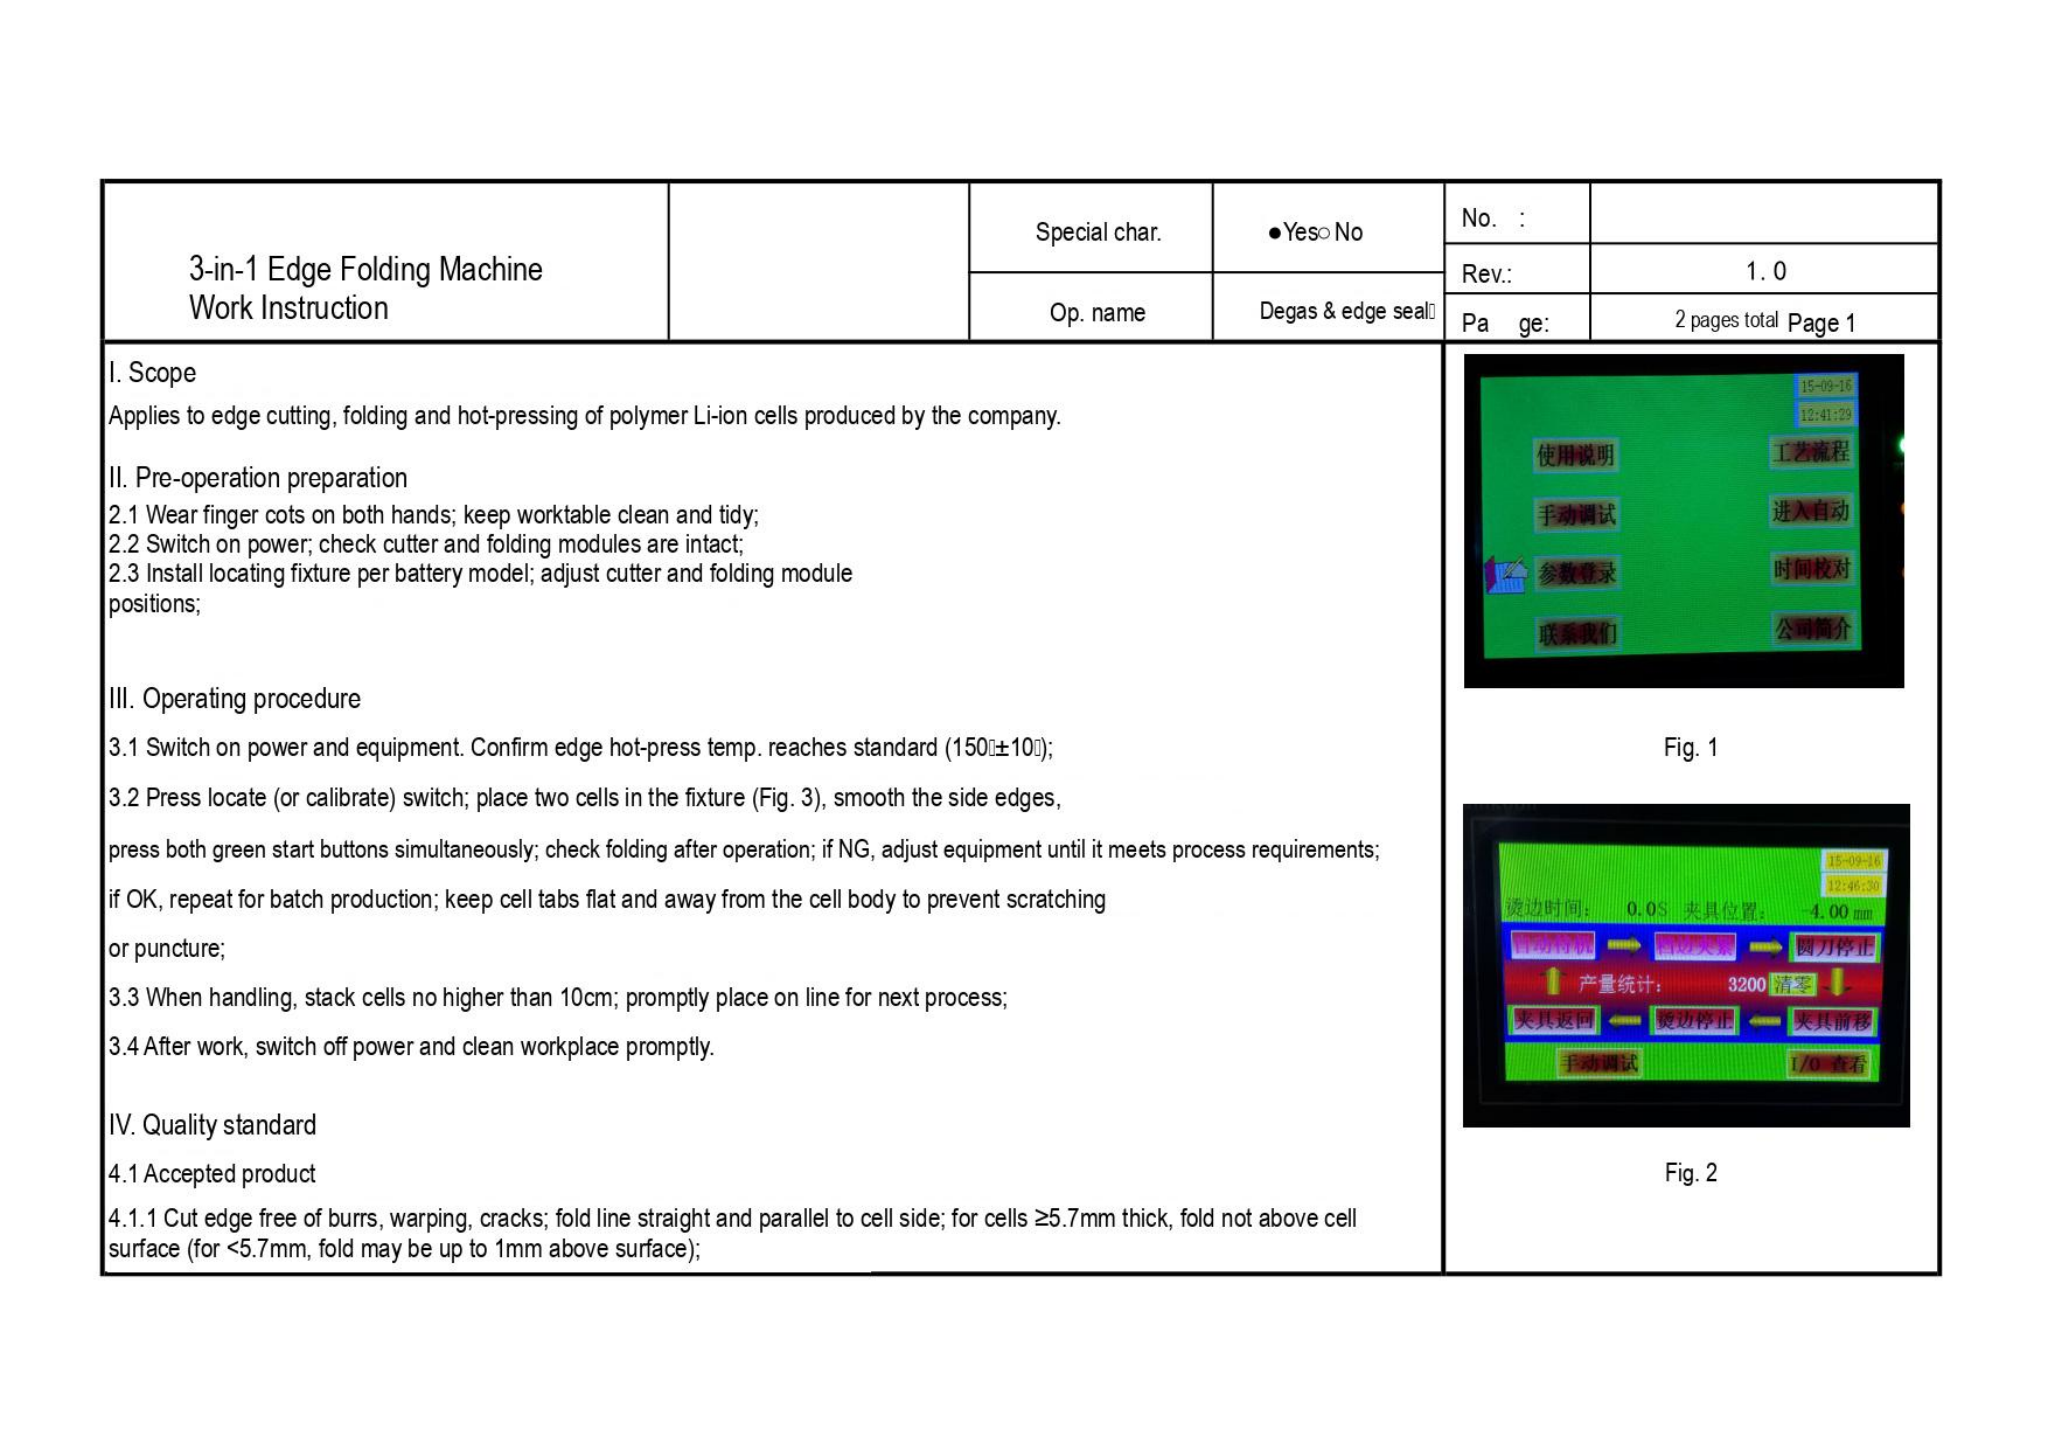| 3-in-1 Edge Folding Machine Work Instruction | | Special char. | ●Yes○No | No. : | |
|---|---|---|---|---|---|
| | | Op. name | Degas & edge seal□ | Rev.: | 1. 0 |
| | | | | Pa ge: | 2 pages total Page 1 |

I. Scope

Applies to edge cutting, folding and hot-pressing of polymer Li-ion cells produced by the company.

II. Pre-operation preparation

2.1 Wear finger cots on both hands; keep worktable clean and tidy;
2.2 Switch on power; check cutter and folding modules are intact;
2.3 Install locating fixture per battery model; adjust cutter and folding module positions;

III. Operating procedure

3.1 Switch on power and equipment. Confirm edge hot-press temp. reaches standard (150□±10□);

3.2 Press locate (or calibrate) switch; place two cells in the fixture (Fig. 3), smooth the side edges,

press both green start buttons simultaneously; check folding after operation; if NG, adjust equipment until it meets process requirements;

if OK, repeat for batch production; keep cell tabs flat and away from the cell body to prevent scratching

or puncture;

3.3 When handling, stack cells no higher than 10cm; promptly place on line for next process;

3.4 After work, switch off power and clean workplace promptly.

IV. Quality standard

4.1 Accepted product

4.1.1 Cut edge free of burrs, warping, cracks; fold line straight and parallel to cell side; for cells ≥5.7mm thick, fold not above cell surface (for <5.7mm, fold may be up to 1mm above surface);

15-09-16
12:41:29
使用说明 工艺流程
手动调试 进入自动
参数登录 时间校对
联系我们 公司简介

Fig. 1

15-09-16
12:46:30
烫边时间: 0.0S 夹具位置: -4.00 mm
圆刀停止
产量统计: 3200 清零
夹具返回 烫边停止 夹具前移
手动调试 I/O 查看

Fig. 2
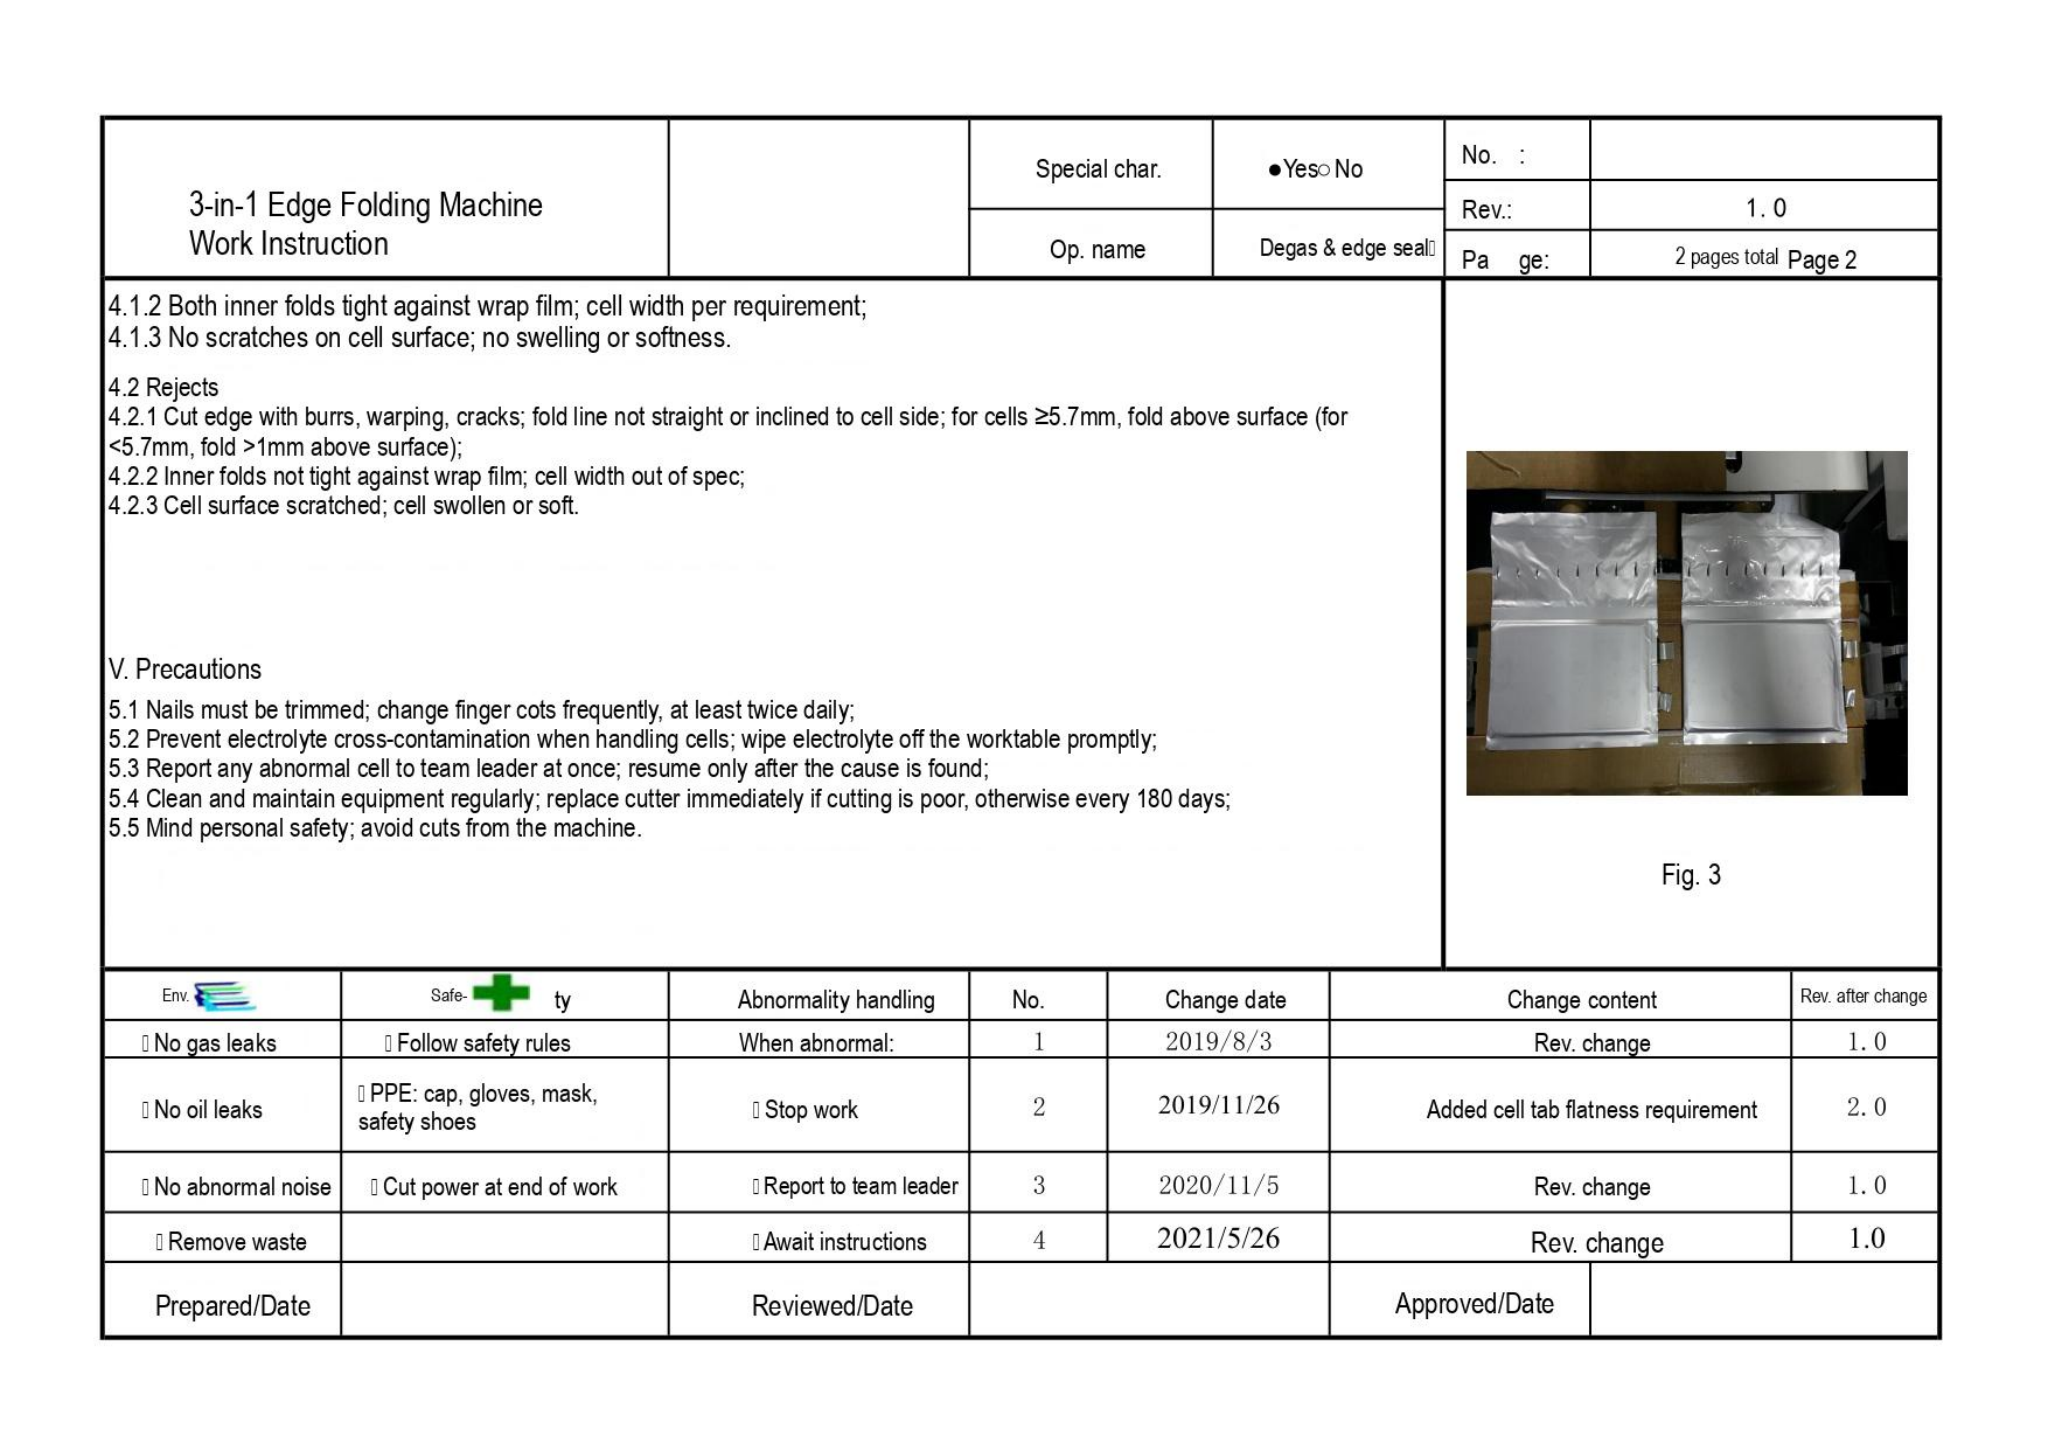| 3-in-1 Edge Folding Machine Work Instruction | | Special char. | ●Yes○No | No. : | |
|---|---|---|---|---|---|
| | | | | Rev.: | 1. 0 |
| | | Op. name | Degas & edge seal | Page: | 2 pages total Page 2 |

4.1.2 Both inner folds tight against wrap film; cell width per requirement;
4.1.3 No scratches on cell surface; no swelling or softness.

4.2 Rejects
4.2.1 Cut edge with burrs, warping, cracks; fold line not straight or inclined to cell side; for cells ≥5.7mm, fold above surface (for <5.7mm, fold >1mm above surface);
4.2.2 Inner folds not tight against wrap film; cell width out of spec;
4.2.3 Cell surface scratched; cell swollen or soft.

V. Precautions
5.1 Nails must be trimmed; change finger cots frequently, at least twice daily;
5.2 Prevent electrolyte cross-contamination when handling cells; wipe electrolyte off the worktable promptly;
5.3 Report any abnormal cell to team leader at once; resume only after the cause is found;
5.4 Clean and maintain equipment regularly; replace cutter immediately if cutting is poor, otherwise every 180 days;
5.5 Mind personal safety; avoid cuts from the machine.

Fig. 3

| Env. | Safety | Abnormality handling | No. | Change date | Change content | Rev. after change |
|---|---|---|---|---|---|---|
| No gas leaks | Follow safety rules | When abnormal: | 1 | 2019/8/3 | Rev. change | 1. 0 |
| No oil leaks | PPE: cap, gloves, mask, safety shoes | Stop work | 2 | 2019/11/26 | Added cell tab flatness requirement | 2. 0 |
| No abnormal noise | Cut power at end of work | Report to team leader | 3 | 2020/11/5 | Rev. change | 1. 0 |
| Remove waste | | Await instructions | 4 | 2021/5/26 | Rev. change | 1.0 |

| Prepared/Date | | Reviewed/Date | | Approved/Date | |
|---|---|---|---|---|---|